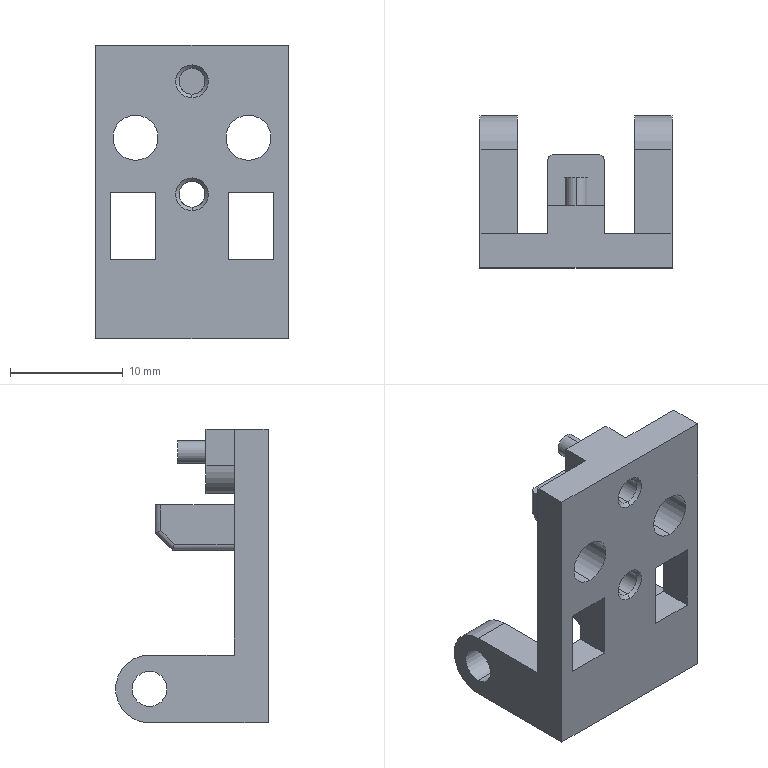Part | STEP file | _X2_751F4E45_X0_MS731-1_X2_8_20 | 1 solid | 56 faces | box 17 x 13.5 x 26 mm | volume 1619 mm3 | plane 29 | cylinder 23 | cone 4 | commonest cylinder face diameters 1 x6 2.3 x4 3.1 x4 4 x4 2 x2 6 x2